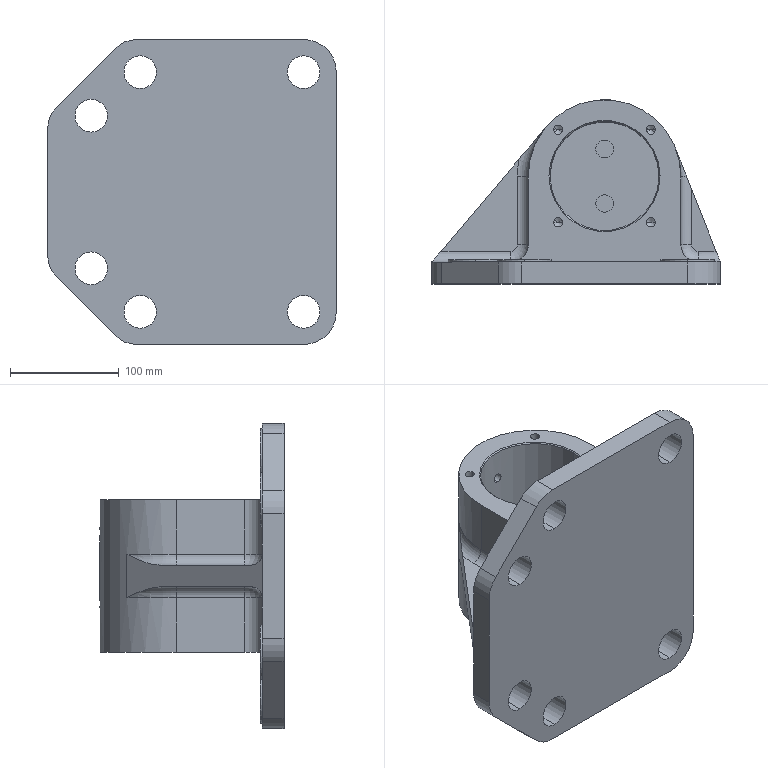Part | SolidWorks | features MirrorStock 1 | 1 solid | 109 faces | box 265 x 169 x 280 mm | volume 3133595 mm3 | cylinder 61 | plane 30 | cone 10 | torus 8 | commonest cylinder face diameters 8.5 x12 30 x12 50 x12 20 x8 60 x6 16 x4